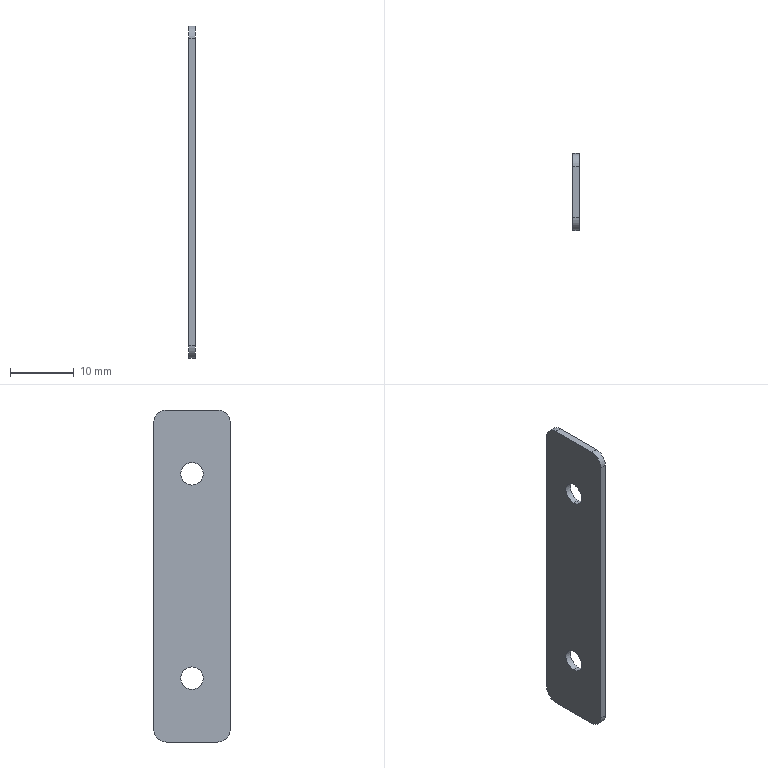Part | STEP file | FFH80-GY-020^FFH85-B3 -02_three-axis module | 1 solid | 14 faces | box 1 x 12 x 52 mm | volume 601.324 mm3 | cylinder 8 | plane 6 | commonest cylinder face diameters 3.5 x4 4 x4
STEP:
#1=CARTESIAN_POINT('',(0.,0.,17.75));
#2=VERTEX_POINT('',#1);
#3=CARTESIAN_POINT('',(0.,0.,14.25));
#4=VERTEX_POINT('',#3);
#5=CARTESIAN_POINT('',(0.,0.,16.));
#6=DIRECTION('',(1.,0.,0.));
#7=DIRECTION('',(0.,0.,-1.));
#8=AXIS2_PLACEMENT_3D('',#5,#6,#7);
#9=CIRCLE('',#8,1.75);
#10=EDGE_CURVE('',#2,#4,#9,.T.);
#11=ORIENTED_EDGE('',*,*,#10,.F.);
#12=CARTESIAN_POINT('',(1.,0.,17.75));
#13=VERTEX_POINT('',#12);
#14=CARTESIAN_POINT('',(1.,0.,17.75));
#15=DIRECTION('',(1.,0.,0.));
#16=VECTOR('',#15,1000.);
#17=LINE('',#14,#16);
#18=EDGE_CURVE('',#2,#13,#17,.T.);
#19=ORIENTED_EDGE('',*,*,#18,.T.);
#20=CARTESIAN_POINT('',(1.,0.,14.25));
#21=VERTEX_POINT('',#20);
#22=CARTESIAN_POINT('',(1.,0.,16.));
#23=DIRECTION('',(-1.,0.,0.));
#24=DIRECTION('',(0.,0.,-1.));
#25=AXIS2_PLACEMENT_3D('',#22,#23,#24);
#26=CIRCLE('',#25,1.75);
#27=EDGE_CURVE('',#21,#13,#26,.T.);
#28=ORIENTED_EDGE('',*,*,#27,.F.);
#29=CARTESIAN_POINT('',(1.,0.,14.25));
#30=DIRECTION('',(1.,0.,0.));
#31=VECTOR('',#30,1000.);
#32=LINE('',#29,#31);
#33=EDGE_CURVE('',#4,#21,#32,.T.);
#34=ORIENTED_EDGE('',*,*,#33,.F.);
#35=EDGE_LOOP('',(#11,#19,#28,#34));
#36=FACE_OUTER_BOUND('',#35,.T.);
#37=CARTESIAN_POINT('',(1.,0.,16.));
#38=DIRECTION('',(1.,0.,0.));
#39=DIRECTION('',(0.,0.,-1.));
#40=AXIS2_PLACEMENT_3D('',#37,#38,#39);
#41=CYLINDRICAL_SURFACE('',#40,1.75);
#42=ADVANCED_FACE('',(#36),#41,.F.);
#43=CARTESIAN_POINT('',(0.,0.,-14.25));
#44=VERTEX_POINT('',#43);
#45=CARTESIAN_POINT('',(0.,0.,-17.75));
#46=VERTEX_POINT('',#45);
#47=CARTESIAN_POINT('',(0.,0.,-16.));
#48=DIRECTION('',(1.,0.,0.));
#49=DIRECTION('',(0.,0.,-1.));
#50=AXIS2_PLACEMENT_3D('',#47,#48,#49);
#51=CIRCLE('',#50,1.75);
#52=EDGE_CURVE('',#44,#46,#51,.T.);
#53=ORIENTED_EDGE('',*,*,#52,.F.);
#54=CARTESIAN_POINT('',(1.,0.,-14.25));
#55=VERTEX_POINT('',#54);
#56=CARTESIAN_POINT('',(1.,0.,-14.25));
#57=DIRECTION('',(1.,0.,0.));
#58=VECTOR('',#57,1000.);
#59=LINE('',#56,#58);
#60=EDGE_CURVE('',#44,#55,#59,.T.);
#61=ORIENTED_EDGE('',*,*,#60,.T.);
#62=CARTESIAN_POINT('',(1.,0.,-17.75));
#63=VERTEX_POINT('',#62);
#64=CARTESIAN_POINT('',(1.,0.,-16.));
#65=DIRECTION('',(-1.,0.,0.));
#66=DIRECTION('',(0.,0.,-1.));
#67=AXIS2_PLACEMENT_3D('',#64,#65,#66);
#68=CIRCLE('',#67,1.75);
#69=EDGE_CURVE('',#63,#55,#68,.T.);
#70=ORIENTED_EDGE('',*,*,#69,.F.);
#71=CARTESIAN_POINT('',(1.,0.,-17.75));
#72=DIRECTION('',(1.,0.,0.));
#73=VECTOR('',#72,1000.);
#74=LINE('',#71,#73);
#75=EDGE_CURVE('',#46,#63,#74,.T.);
#76=ORIENTED_EDGE('',*,*,#75,.F.);
#77=EDGE_LOOP('',(#53,#61,#70,#76));
#78=FACE_OUTER_BOUND('',#77,.T.);
#79=CARTESIAN_POINT('',(1.,0.,-16.));
#80=DIRECTION('',(1.,0.,0.));
#81=DIRECTION('',(0.,0.,-1.));
#82=AXIS2_PLACEMENT_3D('',#79,#80,#81);
#83=CYLINDRICAL_SURFACE('',#82,1.75);
#84=ADVANCED_FACE('',(#78),#83,.F.);
#85=CARTESIAN_POINT('',(0.,0.,16.));
#86=DIRECTION('',(1.,0.,0.));
#87=DIRECTION('',(0.,0.,-1.));
#88=AXIS2_PLACEMENT_3D('',#85,#86,#87);
#89=CIRCLE('',#88,1.75);
#90=EDGE_CURVE('',#4,#2,#89,.T.);
#91=ORIENTED_EDGE('',*,*,#90,.T.);
#92=ORIENTED_EDGE('',*,*,#10,.T.);
#93=EDGE_LOOP('',(#91,#92));
#94=FACE_BOUND('',#93,.T.);
#95=CARTESIAN_POINT('',(0.,0.,-16.));
#96=DIRECTION('',(1.,0.,0.));
#97=DIRECTION('',(0.,0.,-1.));
#98=AXIS2_PLACEMENT_3D('',#95,#96,#97);
#99=CIRCLE('',#98,1.75);
#100=EDGE_CURVE('',#46,#44,#99,.T.);
#101=ORIENTED_EDGE('',*,*,#100,.T.);
#102=ORIENTED_EDGE('',*,*,#52,.T.);
#103=EDGE_LOOP('',(#101,#102));
#104=FACE_BOUND('',#103,.T.);
#105=CARTESIAN_POINT('',(0.,-6.,-24.));
#106=VERTEX_POINT('',#105);
#107=CARTESIAN_POINT('',(0.,-6.,24.));
#108=VERTEX_POINT('',#107);
#109=CARTESIAN_POINT('',(0.,-6.,0.));
#110=DIRECTION('',(0.,0.,1.));
#111=VECTOR('',#110,1000.);
#112=LINE('',#109,#111);
#113=EDGE_CURVE('',#106,#108,#112,.T.);
#114=ORIENTED_EDGE('',*,*,#113,.T.);
#115=CARTESIAN_POINT('',(0.,-4.,26.));
#116=VERTEX_POINT('',#115);
#117=CARTESIAN_POINT('',(0.,-4.,24.));
#118=DIRECTION('',(-1.,0.,0.));
#119=DIRECTION('',(0.,0.,1.));
#120=AXIS2_PLACEMENT_3D('',#117,#118,#119);
#121=CIRCLE('',#120,2.);
#122=EDGE_CURVE('',#108,#116,#121,.T.);
#123=ORIENTED_EDGE('',*,*,#122,.T.);
#124=CARTESIAN_POINT('',(0.,4.,26.));
#125=VERTEX_POINT('',#124);
#126=CARTESIAN_POINT('',(0.,0.,26.));
#127=DIRECTION('',(0.,1.,0.));
#128=VECTOR('',#127,1000.);
#129=LINE('',#126,#128);
#130=EDGE_CURVE('',#116,#125,#129,.T.);
#131=ORIENTED_EDGE('',*,*,#130,.T.);
#132=CARTESIAN_POINT('',(0.,6.,24.));
#133=VERTEX_POINT('',#132);
#134=CARTESIAN_POINT('',(0.,4.,24.));
#135=DIRECTION('',(-1.,0.,0.));
#136=DIRECTION('',(0.,0.,1.));
#137=AXIS2_PLACEMENT_3D('',#134,#135,#136);
#138=CIRCLE('',#137,2.);
#139=EDGE_CURVE('',#125,#133,#138,.T.);
#140=ORIENTED_EDGE('',*,*,#139,.T.);
#141=CARTESIAN_POINT('',(0.,6.,-24.));
#142=VERTEX_POINT('',#141);
#143=CARTESIAN_POINT('',(0.,6.,0.));
#144=DIRECTION('',(0.,0.,-1.));
#145=VECTOR('',#144,1000.);
#146=LINE('',#143,#145);
#147=EDGE_CURVE('',#133,#142,#146,.T.);
#148=ORIENTED_EDGE('',*,*,#147,.T.);
#149=CARTESIAN_POINT('',(0.,4.,-26.));
#150=VERTEX_POINT('',#149);
#151=CARTESIAN_POINT('',(0.,4.,-24.));
#152=DIRECTION('',(-1.,0.,0.));
#153=DIRECTION('',(0.,0.,1.));
#154=AXIS2_PLACEMENT_3D('',#151,#152,#153);
#155=CIRCLE('',#154,2.);
#156=EDGE_CURVE('',#142,#150,#155,.T.);
#157=ORIENTED_EDGE('',*,*,#156,.T.);
#158=CARTESIAN_POINT('',(0.,-4.,-26.));
#159=VERTEX_POINT('',#158);
#160=CARTESIAN_POINT('',(0.,0.,-26.));
#161=DIRECTION('',(0.,-1.,0.));
#162=VECTOR('',#161,1000.);
#163=LINE('',#160,#162);
#164=EDGE_CURVE('',#150,#159,#163,.T.);
#165=ORIENTED_EDGE('',*,*,#164,.T.);
#166=CARTESIAN_POINT('',(0.,-4.,-24.));
#167=DIRECTION('',(-1.,0.,0.));
#168=DIRECTION('',(0.,0.,1.));
#169=AXIS2_PLACEMENT_3D('',#166,#167,#168);
#170=CIRCLE('',#169,2.);
#171=EDGE_CURVE('',#159,#106,#170,.T.);
#172=ORIENTED_EDGE('',*,*,#171,.T.);
#173=EDGE_LOOP('',(#114,#123,#131,#140,#148,#157,#165,#172));
#174=FACE_OUTER_BOUND('',#173,.T.);
#175=CARTESIAN_POINT('',(0.,0.,0.));
#176=DIRECTION('',(-1.,0.,0.));
#177=DIRECTION('',(0.,0.,1.));
#178=AXIS2_PLACEMENT_3D('',#175,#176,#177);
#179=PLANE('',#178);
#180=ADVANCED_FACE('',(#94,#104,#174),#179,.T.);
#181=ORIENTED_EDGE('',*,*,#18,.F.);
#182=ORIENTED_EDGE('',*,*,#90,.F.);
#183=ORIENTED_EDGE('',*,*,#33,.T.);
#184=CARTESIAN_POINT('',(1.,0.,16.));
#185=DIRECTION('',(-1.,0.,0.));
#186=DIRECTION('',(0.,0.,-1.));
#187=AXIS2_PLACEMENT_3D('',#184,#185,#186);
#188=CIRCLE('',#187,1.75);
#189=EDGE_CURVE('',#13,#21,#188,.T.);
#190=ORIENTED_EDGE('',*,*,#189,.F.);
#191=EDGE_LOOP('',(#181,#182,#183,#190));
#192=FACE_OUTER_BOUND('',#191,.T.);
#193=CARTESIAN_POINT('',(1.,0.,16.));
#194=DIRECTION('',(1.,0.,0.));
#195=DIRECTION('',(0.,0.,-1.));
#196=AXIS2_PLACEMENT_3D('',#193,#194,#195);
#197=CYLINDRICAL_SURFACE('',#196,1.75);
#198=ADVANCED_FACE('',(#192),#197,.F.);
#199=ORIENTED_EDGE('',*,*,#60,.F.);
#200=ORIENTED_EDGE('',*,*,#100,.F.);
#201=ORIENTED_EDGE('',*,*,#75,.T.);
#202=CARTESIAN_POINT('',(1.,0.,-16.));
#203=DIRECTION('',(-1.,0.,0.));
#204=DIRECTION('',(0.,0.,-1.));
#205=AXIS2_PLACEMENT_3D('',#202,#203,#204);
#206=CIRCLE('',#205,1.75);
#207=EDGE_CURVE('',#55,#63,#206,.T.);
#208=ORIENTED_EDGE('',*,*,#207,.F.);
#209=EDGE_LOOP('',(#199,#200,#201,#208));
#210=FACE_OUTER_BOUND('',#209,.T.);
#211=CARTESIAN_POINT('',(1.,0.,-16.));
#212=DIRECTION('',(1.,0.,0.));
#213=DIRECTION('',(0.,0.,-1.));
#214=AXIS2_PLACEMENT_3D('',#211,#212,#213);
#215=CYLINDRICAL_SURFACE('',#214,1.75);
#216=ADVANCED_FACE('',(#210),#215,.F.);
#217=CARTESIAN_POINT('',(1.,-6.,24.));
#218=VERTEX_POINT('',#217);
#219=CARTESIAN_POINT('',(1.,-4.,26.));
#220=VERTEX_POINT('',#219);
#221=CARTESIAN_POINT('',(1.,-4.,24.));
#222=DIRECTION('',(-1.,0.,0.));
#223=DIRECTION('',(0.,0.,1.));
#224=AXIS2_PLACEMENT_3D('',#221,#222,#223);
#225=CIRCLE('',#224,2.);
#226=EDGE_CURVE('',#218,#220,#225,.T.);
#227=ORIENTED_EDGE('',*,*,#226,.T.);
#228=CARTESIAN_POINT('',(1.,-4.,26.));
#229=DIRECTION('',(-1.,0.,0.));
#230=VECTOR('',#229,1000.);
#231=LINE('',#228,#230);
#232=EDGE_CURVE('',#220,#116,#231,.T.);
#233=ORIENTED_EDGE('',*,*,#232,.T.);
#234=ORIENTED_EDGE('',*,*,#122,.F.);
#235=CARTESIAN_POINT('',(1.,-6.,24.));
#236=DIRECTION('',(1.,0.,0.));
#237=VECTOR('',#236,1000.);
#238=LINE('',#235,#237);
#239=EDGE_CURVE('',#108,#218,#238,.T.);
#240=ORIENTED_EDGE('',*,*,#239,.T.);
#241=EDGE_LOOP('',(#227,#233,#234,#240));
#242=FACE_OUTER_BOUND('',#241,.T.);
#243=CARTESIAN_POINT('',(1.,-4.,24.));
#244=DIRECTION('',(-1.,0.,0.));
#245=DIRECTION('',(0.,0.,1.));
#246=AXIS2_PLACEMENT_3D('',#243,#244,#245);
#247=CYLINDRICAL_SURFACE('',#246,2.);
#248=ADVANCED_FACE('',(#242),#247,.T.);
#249=CARTESIAN_POINT('',(1.,-6.,-24.));
#250=VERTEX_POINT('',#249);
#251=CARTESIAN_POINT('',(1.,-6.,-26.));
#252=DIRECTION('',(0.,0.,-1.));
#253=VECTOR('',#252,1000.);
#254=LINE('',#251,#253);
#255=EDGE_CURVE('',#218,#250,#254,.T.);
#256=ORIENTED_EDGE('',*,*,#255,.F.);
#257=ORIENTED_EDGE('',*,*,#239,.F.);
#258=ORIENTED_EDGE('',*,*,#113,.F.);
#259=CARTESIAN_POINT('',(1.,-6.,-24.));
#260=DIRECTION('',(-1.,0.,0.));
#261=VECTOR('',#260,1000.);
#262=LINE('',#259,#261);
#263=EDGE_CURVE('',#250,#106,#262,.T.);
#264=ORIENTED_EDGE('',*,*,#263,.F.);
#265=EDGE_LOOP('',(#256,#257,#258,#264));
#266=FACE_OUTER_BOUND('',#265,.T.);
#267=CARTESIAN_POINT('',(1.,-6.,-26.));
#268=DIRECTION('',(0.,1.,0.));
#269=DIRECTION('',(0.,0.,1.));
#270=AXIS2_PLACEMENT_3D('',#267,#268,#269);
#271=PLANE('',#270);
#272=ADVANCED_FACE('',(#266),#271,.F.);
#273=CARTESIAN_POINT('',(1.,-4.,-26.));
#274=VERTEX_POINT('',#273);
#275=CARTESIAN_POINT('',(1.,-4.,-24.));
#276=DIRECTION('',(-1.,0.,0.));
#277=DIRECTION('',(0.,0.,1.));
#278=AXIS2_PLACEMENT_3D('',#275,#276,#277);
#279=CIRCLE('',#278,2.);
#280=EDGE_CURVE('',#274,#250,#279,.T.);
#281=ORIENTED_EDGE('',*,*,#280,.T.);
#282=ORIENTED_EDGE('',*,*,#263,.T.);
#283=ORIENTED_EDGE('',*,*,#171,.F.);
#284=CARTESIAN_POINT('',(1.,-4.,-26.));
#285=DIRECTION('',(1.,0.,0.));
#286=VECTOR('',#285,1000.);
#287=LINE('',#284,#286);
#288=EDGE_CURVE('',#159,#274,#287,.T.);
#289=ORIENTED_EDGE('',*,*,#288,.T.);
#290=EDGE_LOOP('',(#281,#282,#283,#289));
#291=FACE_OUTER_BOUND('',#290,.T.);
#292=CARTESIAN_POINT('',(1.,-4.,-24.));
#293=DIRECTION('',(-1.,0.,0.));
#294=DIRECTION('',(0.,0.,1.));
#295=AXIS2_PLACEMENT_3D('',#292,#293,#294);
#296=CYLINDRICAL_SURFACE('',#295,2.);
#297=ADVANCED_FACE('',(#291),#296,.T.);
#298=CARTESIAN_POINT('',(1.,4.,-26.));
#299=VERTEX_POINT('',#298);
#300=CARTESIAN_POINT('',(1.,6.,-26.));
#301=DIRECTION('',(0.,1.,0.));
#302=VECTOR('',#301,1000.);
#303=LINE('',#300,#302);
#304=EDGE_CURVE('',#274,#299,#303,.T.);
#305=ORIENTED_EDGE('',*,*,#304,.F.);
#306=ORIENTED_EDGE('',*,*,#288,.F.);
#307=ORIENTED_EDGE('',*,*,#164,.F.);
#308=CARTESIAN_POINT('',(1.,4.,-26.));
#309=DIRECTION('',(-1.,0.,0.));
#310=VECTOR('',#309,1000.);
#311=LINE('',#308,#310);
#312=EDGE_CURVE('',#299,#150,#311,.T.);
#313=ORIENTED_EDGE('',*,*,#312,.F.);
#314=EDGE_LOOP('',(#305,#306,#307,#313));
#315=FACE_OUTER_BOUND('',#314,.T.);
#316=CARTESIAN_POINT('',(1.,6.,-26.));
#317=DIRECTION('',(0.,0.,1.));
#318=DIRECTION('',(0.,-1.,0.));
#319=AXIS2_PLACEMENT_3D('',#316,#317,#318);
#320=PLANE('',#319);
#321=ADVANCED_FACE('',(#315),#320,.F.);
#322=CARTESIAN_POINT('',(1.,6.,-24.));
#323=VERTEX_POINT('',#322);
#324=CARTESIAN_POINT('',(1.,4.,-24.));
#325=DIRECTION('',(-1.,0.,0.));
#326=DIRECTION('',(0.,0.,1.));
#327=AXIS2_PLACEMENT_3D('',#324,#325,#326);
#328=CIRCLE('',#327,2.);
#329=EDGE_CURVE('',#323,#299,#328,.T.);
#330=ORIENTED_EDGE('',*,*,#329,.T.);
#331=ORIENTED_EDGE('',*,*,#312,.T.);
#332=ORIENTED_EDGE('',*,*,#156,.F.);
#333=CARTESIAN_POINT('',(1.,6.,-24.));
#334=DIRECTION('',(1.,0.,0.));
#335=VECTOR('',#334,1000.);
#336=LINE('',#333,#335);
#337=EDGE_CURVE('',#142,#323,#336,.T.);
#338=ORIENTED_EDGE('',*,*,#337,.T.);
#339=EDGE_LOOP('',(#330,#331,#332,#338));
#340=FACE_OUTER_BOUND('',#339,.T.);
#341=CARTESIAN_POINT('',(1.,4.,-24.));
#342=DIRECTION('',(-1.,0.,0.));
#343=DIRECTION('',(0.,0.,1.));
#344=AXIS2_PLACEMENT_3D('',#341,#342,#343);
#345=CYLINDRICAL_SURFACE('',#344,2.);
#346=ADVANCED_FACE('',(#340),#345,.T.);
#347=ORIENTED_EDGE('',*,*,#147,.F.);
#348=CARTESIAN_POINT('',(1.,6.,24.));
#349=VERTEX_POINT('',#348);
#350=CARTESIAN_POINT('',(1.,6.,24.));
#351=DIRECTION('',(-1.,0.,0.));
#352=VECTOR('',#351,1000.);
#353=LINE('',#350,#352);
#354=EDGE_CURVE('',#349,#133,#353,.T.);
#355=ORIENTED_EDGE('',*,*,#354,.F.);
#356=CARTESIAN_POINT('',(1.,6.,-26.));
#357=DIRECTION('',(0.,0.,1.));
#358=VECTOR('',#357,1000.);
#359=LINE('',#356,#358);
#360=EDGE_CURVE('',#323,#349,#359,.T.);
#361=ORIENTED_EDGE('',*,*,#360,.F.);
#362=ORIENTED_EDGE('',*,*,#337,.F.);
#363=EDGE_LOOP('',(#347,#355,#361,#362));
#364=FACE_OUTER_BOUND('',#363,.T.);
#365=CARTESIAN_POINT('',(1.,6.,-26.));
#366=DIRECTION('',(0.,-1.,0.));
#367=DIRECTION('',(0.,0.,-1.));
#368=AXIS2_PLACEMENT_3D('',#365,#366,#367);
#369=PLANE('',#368);
#370=ADVANCED_FACE('',(#364),#369,.F.);
#371=CARTESIAN_POINT('',(1.,4.,26.));
#372=VERTEX_POINT('',#371);
#373=CARTESIAN_POINT('',(1.,4.,24.));
#374=DIRECTION('',(-1.,0.,0.));
#375=DIRECTION('',(0.,0.,1.));
#376=AXIS2_PLACEMENT_3D('',#373,#374,#375);
#377=CIRCLE('',#376,2.);
#378=EDGE_CURVE('',#372,#349,#377,.T.);
#379=ORIENTED_EDGE('',*,*,#378,.T.);
#380=ORIENTED_EDGE('',*,*,#354,.T.);
#381=ORIENTED_EDGE('',*,*,#139,.F.);
#382=CARTESIAN_POINT('',(1.,4.,26.));
#383=DIRECTION('',(1.,0.,0.));
#384=VECTOR('',#383,1000.);
#385=LINE('',#382,#384);
#386=EDGE_CURVE('',#125,#372,#385,.T.);
#387=ORIENTED_EDGE('',*,*,#386,.T.);
#388=EDGE_LOOP('',(#379,#380,#381,#387));
#389=FACE_OUTER_BOUND('',#388,.T.);
#390=CARTESIAN_POINT('',(1.,4.,24.));
#391=DIRECTION('',(-1.,0.,0.));
#392=DIRECTION('',(0.,0.,1.));
#393=AXIS2_PLACEMENT_3D('',#390,#391,#392);
#394=CYLINDRICAL_SURFACE('',#393,2.);
#395=ADVANCED_FACE('',(#389),#394,.T.);
#396=CARTESIAN_POINT('',(1.,6.,26.));
#397=DIRECTION('',(0.,-1.,0.));
#398=VECTOR('',#397,1000.);
#399=LINE('',#396,#398);
#400=EDGE_CURVE('',#372,#220,#399,.T.);
#401=ORIENTED_EDGE('',*,*,#400,.F.);
#402=ORIENTED_EDGE('',*,*,#386,.F.);
#403=ORIENTED_EDGE('',*,*,#130,.F.);
#404=ORIENTED_EDGE('',*,*,#232,.F.);
#405=EDGE_LOOP('',(#401,#402,#403,#404));
#406=FACE_OUTER_BOUND('',#405,.T.);
#407=CARTESIAN_POINT('',(1.,6.,26.));
#408=DIRECTION('',(0.,0.,-1.));
#409=DIRECTION('',(-1.,0.,0.));
#410=AXIS2_PLACEMENT_3D('',#407,#408,#409);
#411=PLANE('',#410);
#412=ADVANCED_FACE('',(#406),#411,.F.);
#413=ORIENTED_EDGE('',*,*,#27,.T.);
#414=ORIENTED_EDGE('',*,*,#189,.T.);
#415=EDGE_LOOP('',(#413,#414));
#416=FACE_BOUND('',#415,.T.);
#417=ORIENTED_EDGE('',*,*,#69,.T.);
#418=ORIENTED_EDGE('',*,*,#207,.T.);
#419=EDGE_LOOP('',(#417,#418));
#420=FACE_BOUND('',#419,.T.);
#421=ORIENTED_EDGE('',*,*,#360,.T.);
#422=ORIENTED_EDGE('',*,*,#378,.F.);
#423=ORIENTED_EDGE('',*,*,#400,.T.);
#424=ORIENTED_EDGE('',*,*,#226,.F.);
#425=ORIENTED_EDGE('',*,*,#255,.T.);
#426=ORIENTED_EDGE('',*,*,#280,.F.);
#427=ORIENTED_EDGE('',*,*,#304,.T.);
#428=ORIENTED_EDGE('',*,*,#329,.F.);
#429=EDGE_LOOP('',(#421,#422,#423,#424,#425,#426,#427,#428));
#430=FACE_OUTER_BOUND('',#429,.T.);
#431=CARTESIAN_POINT('',(1.,0.,0.));
#432=DIRECTION('',(-1.,0.,0.));
#433=DIRECTION('',(0.,0.,1.));
#434=AXIS2_PLACEMENT_3D('',#431,#432,#433);
#435=PLANE('',#434);
#436=ADVANCED_FACE('',(#416,#420,#430),#435,.F.);
#437=CLOSED_SHELL('',(#42,#84,#180,#198,#216,#248,#272,#297,#321,#346,#370,#395,#412,#436));
#438=MANIFOLD_SOLID_BREP('',#437);
#439=CARTESIAN_POINT('',(0.,0.,0.));
#440=DIRECTION('',(0.,0.,1.));
#441=DIRECTION('',(1.,0.,0.));
#442=AXIS2_PLACEMENT_3D('',#439,#440,#441);
#443=(LENGTH_UNIT()NAMED_UNIT(*)SI_UNIT(.MILLI.,.METRE.));
#444=UNCERTAINTY_MEASURE_WITH_UNIT(LENGTH_MEASURE(0.00001),#443,'','');
#445=(NAMED_UNIT(*)PLANE_ANGLE_UNIT()SI_UNIT($,.RADIAN.));
#446=(NAMED_UNIT(*)SI_UNIT($,.STERADIAN.)SOLID_ANGLE_UNIT());
#447=(GEOMETRIC_REPRESENTATION_CONTEXT(3)GLOBAL_UNCERTAINTY_ASSIGNED_CONTEXT((#444))GLOBAL_UNIT_ASSIGNED_CONTEXT((#443,#445,#446))REPRESENTATION_CONTEXT('',''));
#448=ADVANCED_BREP_SHAPE_REPRESENTATION('',(#438,#442),#447);